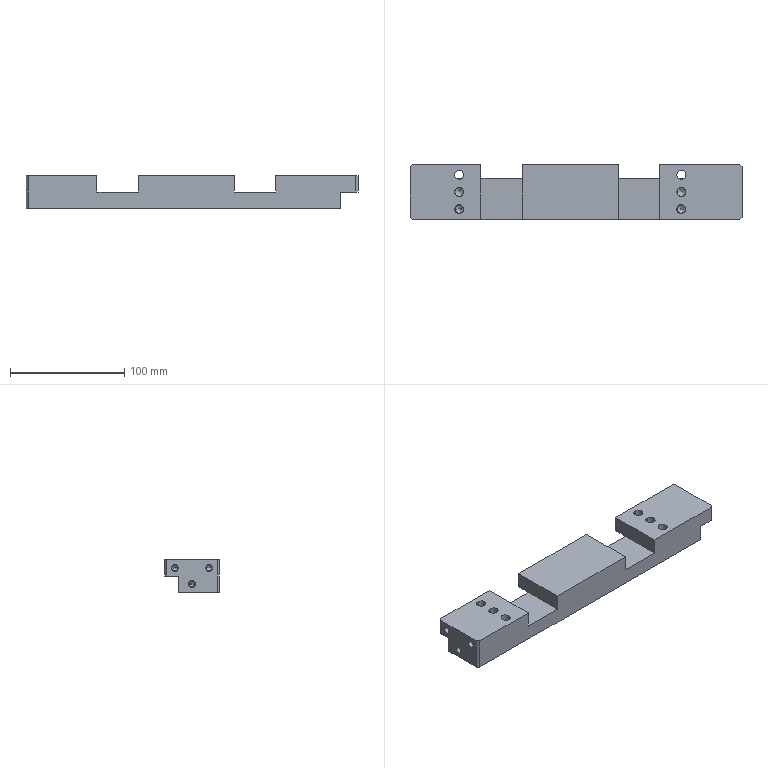Part | STEP file | J454-EBZ05-25-00-Part-1-3 | 1 solid | 129 faces | box 290 x 48 x 28 mm | volume 276441 mm3 | cylinder 60 | plane 41 | cone 28 | commonest cylinder face diameters 6 x14 8 x12 5.1 x10 4.2 x6 5 x6 5.5 x4